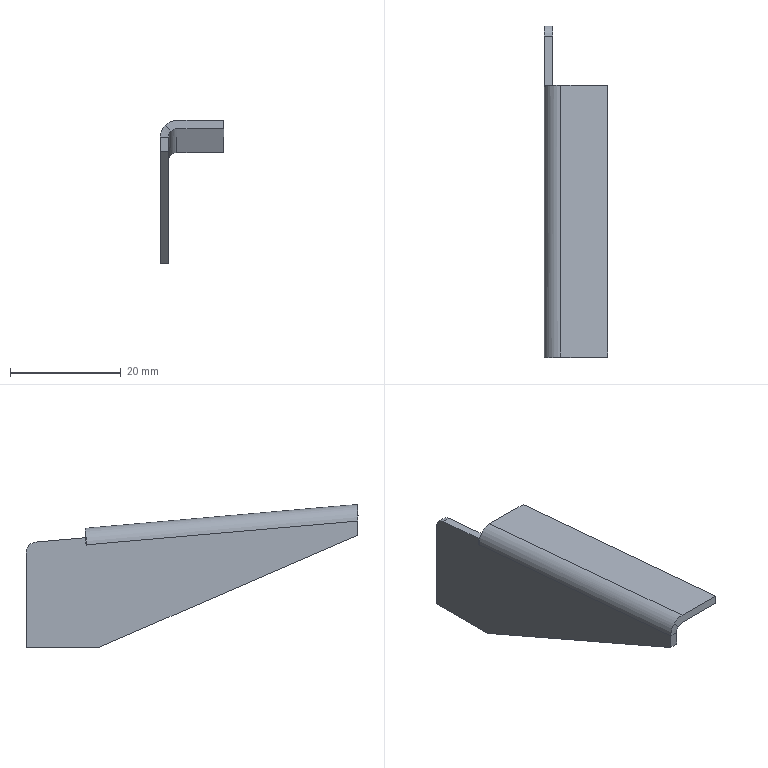Part | NX | features solid 2 | 1 solid | 18 faces | box 11.5 x 60.051 x 25.87 mm | volume 2020 mm3 | plane 14 | cylinder 3 | spline 1 | commonest cylinder face diameters 3 x1 4 x1 6 x1
STEP:
#1=CARTESIAN_POINT('',(166.75,-1519.5,111.869));
#2=VERTEX_POINT('',#1);
#3=CARTESIAN_POINT('',(166.75,-1470.467,107.579));
#4=VERTEX_POINT('',#3);
#5=CARTESIAN_POINT('',(166.75,-1519.5,111.869));
#6=DIRECTION('',(0.,0.9962,-0.08716));
#7=VECTOR('',#6,1000.);
#8=LINE('',#5,#7);
#9=EDGE_CURVE('',#2,#4,#8,.T.);
#10=ORIENTED_EDGE('',*,*,#9,.T.);
#11=CARTESIAN_POINT('',(168.25,-1470.337,109.074));
#12=VERTEX_POINT('',#11);
#13=CARTESIAN_POINT('',(168.25,-1470.467,107.579));
#14=DIRECTION('',(0.,-0.9962,0.08716));
#15=DIRECTION('',(0.,-0.08716,-0.9962));
#16=AXIS2_PLACEMENT_3D('',#13,#14,#15);
#17=CIRCLE('',#16,1.5);
#18=EDGE_CURVE('',#12,#4,#17,.T.);
#19=ORIENTED_EDGE('',*,*,#18,.F.);
#20=CARTESIAN_POINT('',(168.25,-1519.513,113.376));
#21=VERTEX_POINT('',#20);
#22=CARTESIAN_POINT('',(168.25,-1470.337,109.074));
#23=DIRECTION('',(0.,-0.9962,0.08716));
#24=VECTOR('',#23,1000.);
#25=LINE('',#22,#24);
#26=EDGE_CURVE('',#12,#21,#25,.T.);
#27=ORIENTED_EDGE('',*,*,#26,.T.);
#28=CARTESIAN_POINT('',(167.189,-1519.551,112.938));
#29=VERTEX_POINT('',#28);
#30=CARTESIAN_POINT('',(168.25,-1519.644,111.882));
#31=DIRECTION('',(0.,0.9962,-0.08716));
#32=DIRECTION('',(-1.,0.,0.));
#33=AXIS2_PLACEMENT_3D('',#30,#31,#32);
#34=CIRCLE('',#33,1.5);
#35=EDGE_CURVE('',#29,#21,#34,.T.);
#36=ORIENTED_EDGE('',*,*,#35,.F.);
#37=CARTESIAN_POINT('',(167.189,-1519.551,112.938));
#38=CARTESIAN_POINT('',(166.912,-1519.528,112.657));
#39=CARTESIAN_POINT('',(166.75,-1519.514,112.264));
#40=CARTESIAN_POINT('',(166.75,-1519.5,111.869));
#41=B_SPLINE_CURVE_WITH_KNOTS('',3,(#37,#38,#39,#40),.UNSPECIFIED.,.F.,.F.,(4,4),(0.,1.),.UNSPECIFIED.);
#42=EDGE_CURVE('',#2,#29,#41,.F.);
#43=ORIENTED_EDGE('',*,*,#42,.F.);
#44=EDGE_LOOP('',(#10,#19,#27,#36,#43));
#45=FACE_BOUND('',#44,.T.);
#46=CARTESIAN_POINT('',(168.25,-1519.5,111.869));
#47=DIRECTION('',(0.,0.9962,-0.08716));
#48=DIRECTION('',(1.,0.,0.));
#49=AXIS2_PLACEMENT_3D('',#46,#47,#48);
#50=CYLINDRICAL_SURFACE('',#49,1.5);
#51=ADVANCED_FACE('',(#45),#50,.F.);
#52=CARTESIAN_POINT('',(165.25,-1519.5,111.869));
#53=VERTEX_POINT('',#52);
#54=CARTESIAN_POINT('',(165.25,-1470.467,107.579));
#55=VERTEX_POINT('',#54);
#56=CARTESIAN_POINT('',(165.25,-1519.5,111.869));
#57=DIRECTION('',(0.,0.9962,-0.08716));
#58=VECTOR('',#57,1000.);
#59=LINE('',#56,#58);
#60=EDGE_CURVE('',#53,#55,#59,.T.);
#61=ORIENTED_EDGE('',*,*,#60,.F.);
#62=CARTESIAN_POINT('',(166.129,-1519.459,113.995));
#63=VERTEX_POINT('',#62);
#64=CARTESIAN_POINT('',(165.25,-1519.5,111.869));
#65=CARTESIAN_POINT('',(165.25,-1519.479,112.656));
#66=CARTESIAN_POINT('',(165.573,-1519.459,113.437));
#67=CARTESIAN_POINT('',(166.129,-1519.459,113.995));
#68=B_SPLINE_CURVE_WITH_KNOTS('',3,(#64,#65,#66,#67),.UNSPECIFIED.,.F.,.F.,(4,4),(0.,1.),.UNSPECIFIED.);
#69=EDGE_CURVE('',#53,#63,#68,.T.);
#70=ORIENTED_EDGE('',*,*,#69,.T.);
#71=CARTESIAN_POINT('',(168.25,-1519.382,114.87));
#72=VERTEX_POINT('',#71);
#73=CARTESIAN_POINT('',(168.25,-1519.644,111.882));
#74=DIRECTION('',(0.,0.9962,-0.08716));
#75=DIRECTION('',(1.,0.,0.));
#76=AXIS2_PLACEMENT_3D('',#73,#74,#75);
#77=CIRCLE('',#76,3.);
#78=EDGE_CURVE('',#63,#72,#77,.T.);
#79=ORIENTED_EDGE('',*,*,#78,.T.);
#80=CARTESIAN_POINT('',(168.25,-1470.206,110.568));
#81=VERTEX_POINT('',#80);
#82=CARTESIAN_POINT('',(168.25,-1470.206,110.568));
#83=DIRECTION('',(0.,-0.9962,0.08716));
#84=VECTOR('',#83,1000.);
#85=LINE('',#82,#84);
#86=EDGE_CURVE('',#81,#72,#85,.T.);
#87=ORIENTED_EDGE('',*,*,#86,.F.);
#88=CARTESIAN_POINT('',(168.25,-1470.467,107.579));
#89=DIRECTION('',(0.,-0.9962,0.08716));
#90=DIRECTION('',(1.,0.,0.));
#91=AXIS2_PLACEMENT_3D('',#88,#89,#90);
#92=CIRCLE('',#91,3.);
#93=EDGE_CURVE('',#81,#55,#92,.T.);
#94=ORIENTED_EDGE('',*,*,#93,.T.);
#95=EDGE_LOOP('',(#61,#70,#79,#87,#94));
#96=FACE_BOUND('',#95,.T.);
#97=CARTESIAN_POINT('',(168.25,-1519.5,111.869));
#98=DIRECTION('',(0.,0.9962,-0.08716));
#99=DIRECTION('',(1.,0.,0.));
#100=AXIS2_PLACEMENT_3D('',#97,#98,#99);
#101=CYLINDRICAL_SURFACE('',#100,3.);
#102=ADVANCED_FACE('',(#96),#101,.T.);
#103=ORIENTED_EDGE('',*,*,#42,.T.);
#104=CARTESIAN_POINT('',(166.129,-1519.459,113.995));
#105=DIRECTION('',(-0.7071,0.06163,0.7044));
#106=VECTOR('',#105,1000.);
#107=LINE('',#104,#106);
#108=EDGE_CURVE('',#29,#63,#107,.T.);
#109=ORIENTED_EDGE('',*,*,#108,.T.);
#110=ORIENTED_EDGE('',*,*,#69,.F.);
#111=CARTESIAN_POINT('',(166.75,-1519.5,111.869));
#112=DIRECTION('',(-1.,0.,0.));
#113=VECTOR('',#112,1000.);
#114=LINE('',#111,#113);
#115=EDGE_CURVE('',#2,#53,#114,.T.);
#116=ORIENTED_EDGE('',*,*,#115,.F.);
#117=EDGE_LOOP('',(#103,#109,#110,#116));
#118=FACE_BOUND('',#117,.T.);
#119=CARTESIAN_POINT('',(165.25,-1519.5,111.869));
#120=CARTESIAN_POINT('',(165.25,-1519.49,112.262));
#121=CARTESIAN_POINT('',(165.328,-1519.479,112.656));
#122=CARTESIAN_POINT('',(165.629,-1519.464,113.383));
#123=CARTESIAN_POINT('',(165.851,-1519.459,113.716));
#124=CARTESIAN_POINT('',(166.129,-1519.459,113.995));
#125=CARTESIAN_POINT('',(166.75,-1519.5,111.869));
#126=CARTESIAN_POINT('',(166.75,-1519.507,112.067));
#127=CARTESIAN_POINT('',(166.789,-1519.514,112.264));
#128=CARTESIAN_POINT('',(166.939,-1519.53,112.63));
#129=CARTESIAN_POINT('',(167.05,-1519.539,112.798));
#130=CARTESIAN_POINT('',(167.189,-1519.551,112.938));
#131=(BOUNDED_SURFACE()B_SPLINE_SURFACE(1,3,((#119,#120,#121,#122,#123,#124),(#125,#126,#127,#128,#129,#130)),.RULED_SURF.,.F.,.F.,.F.)B_SPLINE_SURFACE_WITH_KNOTS((2,2),(4,2,4),(0.,1.),(0.,0.5,1.),.UNSPECIFIED.)GEOMETRIC_REPRESENTATION_ITEM()RATIONAL_B_SPLINE_SURFACE(((1.,1.,1.,1.,1.,1.),(1.,1.,1.,1.,1.,1.)))REPRESENTATION_ITEM('')SURFACE());
#132=ADVANCED_FACE('',(#118),#131,.T.);
#133=CARTESIAN_POINT('',(176.75,-1519.513,113.376));
#134=VERTEX_POINT('',#133);
#135=CARTESIAN_POINT('',(176.75,-1470.337,109.074));
#136=VERTEX_POINT('',#135);
#137=CARTESIAN_POINT('',(176.75,-1519.513,113.376));
#138=DIRECTION('',(0.,0.9962,-0.08716));
#139=VECTOR('',#138,1000.);
#140=LINE('',#137,#139);
#141=EDGE_CURVE('',#134,#136,#140,.T.);
#142=ORIENTED_EDGE('',*,*,#141,.T.);
#143=CARTESIAN_POINT('',(176.75,-1470.206,110.568));
#144=VERTEX_POINT('',#143);
#145=CARTESIAN_POINT('',(176.75,-1470.206,110.568));
#146=DIRECTION('',(0.,-0.08716,-0.9962));
#147=VECTOR('',#146,1000.);
#148=LINE('',#145,#147);
#149=EDGE_CURVE('',#144,#136,#148,.T.);
#150=ORIENTED_EDGE('',*,*,#149,.F.);
#151=CARTESIAN_POINT('',(176.75,-1519.382,114.87));
#152=VERTEX_POINT('',#151);
#153=CARTESIAN_POINT('',(176.75,-1519.382,114.87));
#154=DIRECTION('',(0.,0.9962,-0.08716));
#155=VECTOR('',#154,1000.);
#156=LINE('',#153,#155);
#157=EDGE_CURVE('',#152,#144,#156,.T.);
#158=ORIENTED_EDGE('',*,*,#157,.F.);
#159=CARTESIAN_POINT('',(176.75,-1519.382,114.87));
#160=DIRECTION('',(0.,-0.08716,-0.9962));
#161=VECTOR('',#160,1000.);
#162=LINE('',#159,#161);
#163=EDGE_CURVE('',#152,#134,#162,.T.);
#164=ORIENTED_EDGE('',*,*,#163,.T.);
#165=EDGE_LOOP('',(#142,#150,#158,#164));
#166=FACE_BOUND('',#165,.T.);
#167=CARTESIAN_POINT('',(176.75,-1519.382,114.87));
#168=DIRECTION('',(-1.,0.,0.));
#169=DIRECTION('',(0.,0.,1.));
#170=AXIS2_PLACEMENT_3D('',#167,#168,#169);
#171=PLANE('',#170);
#172=ADVANCED_FACE('',(#166),#171,.F.);
#173=ORIENTED_EDGE('',*,*,#26,.F.);
#174=CARTESIAN_POINT('',(166.601,-1470.337,109.074));
#175=DIRECTION('',(-1.,0.,0.));
#176=VECTOR('',#175,1000.);
#177=LINE('',#174,#176);
#178=EDGE_CURVE('',#136,#12,#177,.T.);
#179=ORIENTED_EDGE('',*,*,#178,.F.);
#180=ORIENTED_EDGE('',*,*,#141,.F.);
#181=CARTESIAN_POINT('',(166.601,-1519.513,113.376));
#182=DIRECTION('',(1.,0.,0.));
#183=VECTOR('',#182,1000.);
#184=LINE('',#181,#183);
#185=EDGE_CURVE('',#21,#134,#184,.T.);
#186=ORIENTED_EDGE('',*,*,#185,.F.);
#187=EDGE_LOOP('',(#173,#179,#180,#186));
#188=FACE_BOUND('',#187,.T.);
#189=CARTESIAN_POINT('',(166.601,-1470.337,109.074));
#190=DIRECTION('',(0.,0.08716,0.9962));
#191=DIRECTION('',(1.,0.,0.));
#192=AXIS2_PLACEMENT_3D('',#189,#190,#191);
#193=PLANE('',#192);
#194=ADVANCED_FACE('',(#188),#193,.F.);
#195=CARTESIAN_POINT('',(166.601,-1470.206,110.568));
#196=DIRECTION('',(-1.,0.,0.));
#197=VECTOR('',#196,1000.);
#198=LINE('',#195,#197);
#199=EDGE_CURVE('',#144,#81,#198,.T.);
#200=ORIENTED_EDGE('',*,*,#199,.T.);
#201=ORIENTED_EDGE('',*,*,#86,.T.);
#202=CARTESIAN_POINT('',(166.601,-1519.382,114.87));
#203=DIRECTION('',(1.,0.,0.));
#204=VECTOR('',#203,1000.);
#205=LINE('',#202,#204);
#206=EDGE_CURVE('',#72,#152,#205,.T.);
#207=ORIENTED_EDGE('',*,*,#206,.T.);
#208=ORIENTED_EDGE('',*,*,#157,.T.);
#209=EDGE_LOOP('',(#200,#201,#207,#208));
#210=FACE_BOUND('',#209,.T.);
#211=CARTESIAN_POINT('',(166.601,-1470.206,110.568));
#212=DIRECTION('',(0.,0.08716,0.9962));
#213=DIRECTION('',(1.,0.,0.));
#214=AXIS2_PLACEMENT_3D('',#211,#212,#213);
#215=PLANE('',#214);
#216=ADVANCED_FACE('',(#210),#215,.T.);
#217=ORIENTED_EDGE('',*,*,#206,.F.);
#218=ORIENTED_EDGE('',*,*,#78,.F.);
#219=ORIENTED_EDGE('',*,*,#108,.F.);
#220=ORIENTED_EDGE('',*,*,#35,.T.);
#221=ORIENTED_EDGE('',*,*,#185,.T.);
#222=ORIENTED_EDGE('',*,*,#163,.F.);
#223=EDGE_LOOP('',(#217,#218,#219,#220,#221,#222));
#224=FACE_BOUND('',#223,.T.);
#225=CARTESIAN_POINT('',(166.601,-1519.382,114.87));
#226=DIRECTION('',(0.,0.9962,-0.08716));
#227=DIRECTION('',(-1.,0.,0.));
#228=AXIS2_PLACEMENT_3D('',#225,#226,#227);
#229=PLANE('',#228);
#230=ADVANCED_FACE('',(#224),#229,.F.);
#231=CARTESIAN_POINT('',(166.75,-1470.376,107.471));
#232=VERTEX_POINT('',#231);
#233=CARTESIAN_POINT('',(165.25,-1470.376,107.471));
#234=VERTEX_POINT('',#233);
#235=CARTESIAN_POINT('',(165.25,-1470.376,107.471));
#236=DIRECTION('',(-1.,0.,0.));
#237=VECTOR('',#236,1000.);
#238=LINE('',#235,#237);
#239=EDGE_CURVE('',#232,#234,#238,.T.);
#240=ORIENTED_EDGE('',*,*,#239,.T.);
#241=CARTESIAN_POINT('',(165.25,-1470.476,107.48));
#242=VERTEX_POINT('',#241);
#243=CARTESIAN_POINT('',(165.25,-1470.376,107.471));
#244=DIRECTION('',(0.,0.9962,-0.08716));
#245=VECTOR('',#244,1000.);
#246=LINE('',#243,#245);
#247=EDGE_CURVE('',#242,#234,#246,.T.);
#248=ORIENTED_EDGE('',*,*,#247,.F.);
#249=CARTESIAN_POINT('',(166.75,-1470.476,107.48));
#250=VERTEX_POINT('',#249);
#251=CARTESIAN_POINT('',(165.25,-1470.476,107.48));
#252=DIRECTION('',(-1.,0.,0.));
#253=VECTOR('',#252,1000.);
#254=LINE('',#251,#253);
#255=EDGE_CURVE('',#250,#242,#254,.T.);
#256=ORIENTED_EDGE('',*,*,#255,.F.);
#257=CARTESIAN_POINT('',(166.75,-1470.376,107.471));
#258=DIRECTION('',(0.,0.9962,-0.08716));
#259=VECTOR('',#258,1000.);
#260=LINE('',#257,#259);
#261=EDGE_CURVE('',#250,#232,#260,.T.);
#262=ORIENTED_EDGE('',*,*,#261,.T.);
#263=EDGE_LOOP('',(#240,#248,#256,#262));
#264=FACE_BOUND('',#263,.T.);
#265=CARTESIAN_POINT('',(165.25,-1470.376,107.471));
#266=DIRECTION('',(0.,-0.08716,-0.9962));
#267=DIRECTION('',(0.,-0.9962,0.08716));
#268=AXIS2_PLACEMENT_3D('',#265,#266,#267);
#269=PLANE('',#268);
#270=ADVANCED_FACE('',(#264),#269,.F.);
#271=CARTESIAN_POINT('',(166.75,-1470.254,108.866));
#272=VERTEX_POINT('',#271);
#273=CARTESIAN_POINT('',(165.25,-1470.254,108.866));
#274=VERTEX_POINT('',#273);
#275=CARTESIAN_POINT('',(166.75,-1470.254,108.866));
#276=DIRECTION('',(-1.,0.,0.));
#277=VECTOR('',#276,1000.);
#278=LINE('',#275,#277);
#279=EDGE_CURVE('',#272,#274,#278,.T.);
#280=ORIENTED_EDGE('',*,*,#279,.T.);
#281=CARTESIAN_POINT('',(165.25,-1470.106,110.559));
#282=DIRECTION('',(0.,0.08716,0.9962));
#283=VECTOR('',#282,1000.);
#284=LINE('',#281,#283);
#285=EDGE_CURVE('',#234,#274,#284,.T.);
#286=ORIENTED_EDGE('',*,*,#285,.F.);
#287=ORIENTED_EDGE('',*,*,#239,.F.);
#288=CARTESIAN_POINT('',(166.75,-1470.106,110.559));
#289=DIRECTION('',(0.,0.08716,0.9962));
#290=VECTOR('',#289,1000.);
#291=LINE('',#288,#290);
#292=EDGE_CURVE('',#232,#272,#291,.T.);
#293=ORIENTED_EDGE('',*,*,#292,.T.);
#294=EDGE_LOOP('',(#280,#286,#287,#293));
#295=FACE_BOUND('',#294,.T.);
#296=CARTESIAN_POINT('',(165.25,-1470.106,110.559));
#297=DIRECTION('',(0.,0.9962,-0.08716));
#298=DIRECTION('',(-1.,0.,0.));
#299=AXIS2_PLACEMENT_3D('',#296,#297,#298);
#300=PLANE('',#299);
#301=ADVANCED_FACE('',(#295),#300,.F.);
#302=ORIENTED_EDGE('',*,*,#9,.F.);
#303=CARTESIAN_POINT('',(166.75,-1519.5,109.3));
#304=VERTEX_POINT('',#303);
#305=CARTESIAN_POINT('',(166.75,-1519.5,109.3));
#306=DIRECTION('',(0.,0.,1.));
#307=VECTOR('',#306,1000.);
#308=LINE('',#305,#307);
#309=EDGE_CURVE('',#304,#2,#308,.T.);
#310=ORIENTED_EDGE('',*,*,#309,.F.);
#311=CARTESIAN_POINT('',(166.75,-1472.655,89.));
#312=VERTEX_POINT('',#311);
#313=CARTESIAN_POINT('',(166.75,-1472.655,89.));
#314=DIRECTION('',(0.,-0.9176,0.3976));
#315=VECTOR('',#314,1000.);
#316=LINE('',#313,#315);
#317=EDGE_CURVE('',#312,#304,#316,.T.);
#318=ORIENTED_EDGE('',*,*,#317,.F.);
#319=CARTESIAN_POINT('',(166.75,-1459.5,89.));
#320=VERTEX_POINT('',#319);
#321=CARTESIAN_POINT('',(166.75,-1472.655,89.));
#322=DIRECTION('',(0.,-1.,0.));
#323=VECTOR('',#322,1000.);
#324=LINE('',#321,#323);
#325=EDGE_CURVE('',#320,#312,#324,.T.);
#326=ORIENTED_EDGE('',*,*,#325,.F.);
#327=CARTESIAN_POINT('',(166.75,-1459.5,106.092));
#328=VERTEX_POINT('',#327);
#329=CARTESIAN_POINT('',(166.75,-1459.5,104.987));
#330=DIRECTION('',(0.,0.,-1.));
#331=VECTOR('',#330,1000.);
#332=LINE('',#329,#331);
#333=EDGE_CURVE('',#328,#320,#332,.T.);
#334=ORIENTED_EDGE('',*,*,#333,.F.);
#335=CARTESIAN_POINT('',(166.75,-1461.326,108.084));
#336=VERTEX_POINT('',#335);
#337=CARTESIAN_POINT('',(166.75,-1461.5,106.092));
#338=DIRECTION('',(-1.,0.,0.));
#339=DIRECTION('',(0.,-1.,0.));
#340=AXIS2_PLACEMENT_3D('',#337,#338,#339);
#341=CIRCLE('',#340,2.);
#342=EDGE_CURVE('',#336,#328,#341,.T.);
#343=ORIENTED_EDGE('',*,*,#342,.F.);
#344=CARTESIAN_POINT('',(166.75,-1461.01,108.057));
#345=DIRECTION('',(0.,0.9962,-0.08716));
#346=VECTOR('',#345,1000.);
#347=LINE('',#344,#346);
#348=EDGE_CURVE('',#272,#336,#347,.T.);
#349=ORIENTED_EDGE('',*,*,#348,.F.);
#350=ORIENTED_EDGE('',*,*,#292,.F.);
#351=ORIENTED_EDGE('',*,*,#261,.F.);
#352=CARTESIAN_POINT('',(166.75,-1470.206,110.568));
#353=DIRECTION('',(0.,-0.08716,-0.9962));
#354=VECTOR('',#353,1000.);
#355=LINE('',#352,#354);
#356=EDGE_CURVE('',#4,#250,#355,.T.);
#357=ORIENTED_EDGE('',*,*,#356,.F.);
#358=EDGE_LOOP('',(#302,#310,#318,#326,#334,#343,#349,#350,#351,#357));
#359=FACE_BOUND('',#358,.T.);
#360=CARTESIAN_POINT('',(166.75,-1461.5,106.092));
#361=DIRECTION('',(-1.,0.,0.));
#362=DIRECTION('',(0.,0.,1.));
#363=AXIS2_PLACEMENT_3D('',#360,#361,#362);
#364=PLANE('',#363);
#365=ADVANCED_FACE('',(#359),#364,.F.);
#366=CARTESIAN_POINT('',(165.25,-1472.655,89.));
#367=VERTEX_POINT('',#366);
#368=CARTESIAN_POINT('',(165.25,-1519.5,109.3));
#369=VERTEX_POINT('',#368);
#370=CARTESIAN_POINT('',(165.25,-1472.655,89.));
#371=DIRECTION('',(0.,-0.9176,0.3976));
#372=VECTOR('',#371,1000.);
#373=LINE('',#370,#372);
#374=EDGE_CURVE('',#367,#369,#373,.T.);
#375=ORIENTED_EDGE('',*,*,#374,.F.);
#376=CARTESIAN_POINT('',(166.75,-1472.655,89.));
#377=DIRECTION('',(-1.,0.,0.));
#378=VECTOR('',#377,1000.);
#379=LINE('',#376,#378);
#380=EDGE_CURVE('',#312,#367,#379,.T.);
#381=ORIENTED_EDGE('',*,*,#380,.F.);
#382=ORIENTED_EDGE('',*,*,#317,.T.);
#383=CARTESIAN_POINT('',(166.75,-1519.5,109.3));
#384=DIRECTION('',(-1.,0.,0.));
#385=VECTOR('',#384,1000.);
#386=LINE('',#383,#385);
#387=EDGE_CURVE('',#304,#369,#386,.T.);
#388=ORIENTED_EDGE('',*,*,#387,.T.);
#389=EDGE_LOOP('',(#375,#381,#382,#388));
#390=FACE_BOUND('',#389,.T.);
#391=CARTESIAN_POINT('',(166.75,-1472.655,89.));
#392=DIRECTION('',(0.,-0.3976,-0.9176));
#393=DIRECTION('',(0.,-0.9176,0.3976));
#394=AXIS2_PLACEMENT_3D('',#391,#392,#393);
#395=PLANE('',#394);
#396=ADVANCED_FACE('',(#390),#395,.T.);
#397=CARTESIAN_POINT('',(165.25,-1459.5,89.));
#398=VERTEX_POINT('',#397);
#399=CARTESIAN_POINT('',(165.25,-1472.655,89.));
#400=DIRECTION('',(0.,-1.,0.));
#401=VECTOR('',#400,1000.);
#402=LINE('',#399,#401);
#403=EDGE_CURVE('',#398,#367,#402,.T.);
#404=ORIENTED_EDGE('',*,*,#403,.F.);
#405=CARTESIAN_POINT('',(166.75,-1459.5,89.));
#406=DIRECTION('',(-1.,0.,0.));
#407=VECTOR('',#406,1000.);
#408=LINE('',#405,#407);
#409=EDGE_CURVE('',#320,#398,#408,.T.);
#410=ORIENTED_EDGE('',*,*,#409,.F.);
#411=ORIENTED_EDGE('',*,*,#325,.T.);
#412=ORIENTED_EDGE('',*,*,#380,.T.);
#413=EDGE_LOOP('',(#404,#410,#411,#412));
#414=FACE_BOUND('',#413,.T.);
#415=CARTESIAN_POINT('',(166.75,-1472.655,89.));
#416=DIRECTION('',(0.,0.,-1.));
#417=DIRECTION('',(0.,-1.,0.));
#418=AXIS2_PLACEMENT_3D('',#415,#416,#417);
#419=PLANE('',#418);
#420=ADVANCED_FACE('',(#414),#419,.T.);
#421=CARTESIAN_POINT('',(165.25,-1459.5,106.092));
#422=VERTEX_POINT('',#421);
#423=CARTESIAN_POINT('',(165.25,-1459.5,104.987));
#424=DIRECTION('',(0.,0.,-1.));
#425=VECTOR('',#424,1000.);
#426=LINE('',#423,#425);
#427=EDGE_CURVE('',#422,#398,#426,.T.);
#428=ORIENTED_EDGE('',*,*,#427,.F.);
#429=CARTESIAN_POINT('',(166.75,-1459.5,106.092));
#430=DIRECTION('',(-1.,0.,0.));
#431=VECTOR('',#430,1000.);
#432=LINE('',#429,#431);
#433=EDGE_CURVE('',#328,#422,#432,.T.);
#434=ORIENTED_EDGE('',*,*,#433,.F.);
#435=ORIENTED_EDGE('',*,*,#333,.T.);
#436=ORIENTED_EDGE('',*,*,#409,.T.);
#437=EDGE_LOOP('',(#428,#434,#435,#436));
#438=FACE_BOUND('',#437,.T.);
#439=CARTESIAN_POINT('',(166.75,-1459.5,104.987));
#440=DIRECTION('',(0.,1.,0.));
#441=DIRECTION('',(1.,0.,0.));
#442=AXIS2_PLACEMENT_3D('',#439,#440,#441);
#443=PLANE('',#442);
#444=ADVANCED_FACE('',(#438),#443,.T.);
#445=CARTESIAN_POINT('',(165.25,-1461.326,108.084));
#446=VERTEX_POINT('',#445);
#447=CARTESIAN_POINT('',(165.25,-1461.5,106.092));
#448=DIRECTION('',(-1.,0.,0.));
#449=DIRECTION('',(0.,-1.,0.));
#450=AXIS2_PLACEMENT_3D('',#447,#448,#449);
#451=CIRCLE('',#450,2.);
#452=EDGE_CURVE('',#446,#422,#451,.T.);
#453=ORIENTED_EDGE('',*,*,#452,.F.);
#454=CARTESIAN_POINT('',(166.75,-1461.326,108.084));
#455=DIRECTION('',(-1.,0.,0.));
#456=VECTOR('',#455,1000.);
#457=LINE('',#454,#456);
#458=EDGE_CURVE('',#336,#446,#457,.T.);
#459=ORIENTED_EDGE('',*,*,#458,.F.);
#460=ORIENTED_EDGE('',*,*,#342,.T.);
#461=ORIENTED_EDGE('',*,*,#433,.T.);
#462=EDGE_LOOP('',(#453,#459,#460,#461));
#463=FACE_BOUND('',#462,.T.);
#464=CARTESIAN_POINT('',(166.75,-1461.5,106.092));
#465=DIRECTION('',(-1.,0.,0.));
#466=DIRECTION('',(0.,0.,-1.));
#467=AXIS2_PLACEMENT_3D('',#464,#465,#466);
#468=CYLINDRICAL_SURFACE('',#467,2.);
#469=ADVANCED_FACE('',(#463),#468,.T.);
#470=ORIENTED_EDGE('',*,*,#279,.F.);
#471=ORIENTED_EDGE('',*,*,#348,.T.);
#472=ORIENTED_EDGE('',*,*,#458,.T.);
#473=CARTESIAN_POINT('',(165.25,-1461.01,108.057));
#474=DIRECTION('',(0.,0.9962,-0.08716));
#475=VECTOR('',#474,1000.);
#476=LINE('',#473,#475);
#477=EDGE_CURVE('',#274,#446,#476,.T.);
#478=ORIENTED_EDGE('',*,*,#477,.F.);
#479=EDGE_LOOP('',(#470,#471,#472,#478));
#480=FACE_BOUND('',#479,.T.);
#481=CARTESIAN_POINT('',(166.75,-1461.01,108.057));
#482=DIRECTION('',(0.,0.08716,0.9962));
#483=DIRECTION('',(1.,0.,0.));
#484=AXIS2_PLACEMENT_3D('',#481,#482,#483);
#485=PLANE('',#484);
#486=ADVANCED_FACE('',(#480),#485,.T.);
#487=CARTESIAN_POINT('',(165.25,-1519.5,109.3));
#488=DIRECTION('',(0.,0.,1.));
#489=VECTOR('',#488,1000.);
#490=LINE('',#487,#489);
#491=EDGE_CURVE('',#369,#53,#490,.T.);
#492=ORIENTED_EDGE('',*,*,#491,.T.);
#493=ORIENTED_EDGE('',*,*,#60,.T.);
#494=CARTESIAN_POINT('',(165.25,-1470.206,110.568));
#495=DIRECTION('',(0.,-0.08716,-0.9962));
#496=VECTOR('',#495,1000.);
#497=LINE('',#494,#496);
#498=EDGE_CURVE('',#55,#242,#497,.T.);
#499=ORIENTED_EDGE('',*,*,#498,.T.);
#500=ORIENTED_EDGE('',*,*,#247,.T.);
#501=ORIENTED_EDGE('',*,*,#285,.T.);
#502=ORIENTED_EDGE('',*,*,#477,.T.);
#503=ORIENTED_EDGE('',*,*,#452,.T.);
#504=ORIENTED_EDGE('',*,*,#427,.T.);
#505=ORIENTED_EDGE('',*,*,#403,.T.);
#506=ORIENTED_EDGE('',*,*,#374,.T.);
#507=EDGE_LOOP('',(#492,#493,#499,#500,#501,#502,#503,#504,#505,#506));
#508=FACE_BOUND('',#507,.T.);
#509=CARTESIAN_POINT('',(165.25,-1461.5,106.092));
#510=DIRECTION('',(-1.,0.,0.));
#511=DIRECTION('',(0.,0.,1.));
#512=AXIS2_PLACEMENT_3D('',#509,#510,#511);
#513=PLANE('',#512);
#514=ADVANCED_FACE('',(#508),#513,.T.);
#515=ORIENTED_EDGE('',*,*,#498,.F.);
#516=ORIENTED_EDGE('',*,*,#93,.F.);
#517=ORIENTED_EDGE('',*,*,#199,.F.);
#518=ORIENTED_EDGE('',*,*,#149,.T.);
#519=ORIENTED_EDGE('',*,*,#178,.T.);
#520=ORIENTED_EDGE('',*,*,#18,.T.);
#521=ORIENTED_EDGE('',*,*,#356,.T.);
#522=ORIENTED_EDGE('',*,*,#255,.T.);
#523=EDGE_LOOP('',(#515,#516,#517,#518,#519,#520,#521,#522));
#524=FACE_BOUND('',#523,.T.);
#525=CARTESIAN_POINT('',(166.75,-1470.206,110.568));
#526=DIRECTION('',(0.,0.9962,-0.08716));
#527=DIRECTION('',(-1.,0.,0.));
#528=AXIS2_PLACEMENT_3D('',#525,#526,#527);
#529=PLANE('',#528);
#530=ADVANCED_FACE('',(#524),#529,.T.);
#531=ORIENTED_EDGE('',*,*,#309,.T.);
#532=ORIENTED_EDGE('',*,*,#115,.T.);
#533=ORIENTED_EDGE('',*,*,#491,.F.);
#534=ORIENTED_EDGE('',*,*,#387,.F.);
#535=EDGE_LOOP('',(#531,#532,#533,#534));
#536=FACE_BOUND('',#535,.T.);
#537=CARTESIAN_POINT('',(166.75,-1519.5,109.3));
#538=DIRECTION('',(0.,-1.,0.));
#539=DIRECTION('',(-1.,0.,0.));
#540=AXIS2_PLACEMENT_3D('',#537,#538,#539);
#541=PLANE('',#540);
#542=ADVANCED_FACE('',(#536),#541,.T.);
#543=CLOSED_SHELL('',(#51,#102,#132,#172,#194,#216,#230,#270,#301,#365,#396,#420,#444,#469,#486,#514,#530,#542));
#544=MANIFOLD_SOLID_BREP('',#543);
#545=(LENGTH_UNIT()NAMED_UNIT(*)SI_UNIT(.MILLI.,.METRE.));
#546=UNCERTAINTY_MEASURE_WITH_UNIT(LENGTH_MEASURE(0.0508),#545,'','');
#547=(NAMED_UNIT(*)PLANE_ANGLE_UNIT()SI_UNIT($,.RADIAN.));
#548=(NAMED_UNIT(*)SI_UNIT($,.STERADIAN.)SOLID_ANGLE_UNIT());
#549=(GEOMETRIC_REPRESENTATION_CONTEXT(3)GLOBAL_UNCERTAINTY_ASSIGNED_CONTEXT((#546))GLOBAL_UNIT_ASSIGNED_CONTEXT((#545,#547,#548))REPRESENTATION_CONTEXT('',''));
#550=ADVANCED_BREP_SHAPE_REPRESENTATION('',(#544),#549);